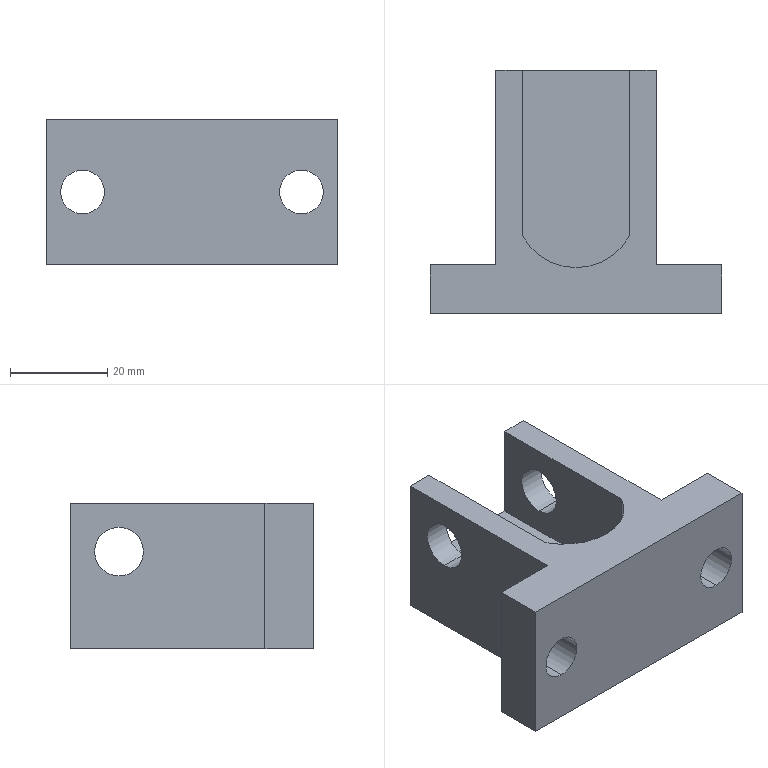Part | SolidWorks | features HoleWzd 3, ICE 3, Extrusion 1 | 1 solid | 22 faces | box 60 x 50 x 30 mm | volume 38448 mm3 | plane 13 | cylinder 9 | commonest cylinder face diameters 9 x4 10 x4 25 x1
STEP:
#1=CARTESIAN_POINT('',(13.5,40.,25.));
#2=VERTEX_POINT('',#1);
#3=CARTESIAN_POINT('',(13.5,40.,15.));
#4=VERTEX_POINT('',#3);
#5=CARTESIAN_POINT('',(13.5,40.,20.));
#6=DIRECTION('',(1.,0.,0.));
#7=DIRECTION('',(0.,1.,0.));
#8=AXIS2_PLACEMENT_3D('',#5,#6,#7);
#9=CIRCLE('',#8,5.);
#10=EDGE_CURVE('',#2,#4,#9,.T.);
#11=ORIENTED_EDGE('',*,*,#10,.F.);
#12=CARTESIAN_POINT('',(19.,40.,25.));
#13=VERTEX_POINT('',#12);
#14=CARTESIAN_POINT('',(19.,40.,25.));
#15=DIRECTION('',(1.,0.,0.));
#16=VECTOR('',#15,1000.);
#17=LINE('',#14,#16);
#18=EDGE_CURVE('',#2,#13,#17,.T.);
#19=ORIENTED_EDGE('',*,*,#18,.T.);
#20=CARTESIAN_POINT('',(19.,40.,15.));
#21=VERTEX_POINT('',#20);
#22=CARTESIAN_POINT('',(19.,40.,20.));
#23=DIRECTION('',(1.,0.,0.));
#24=DIRECTION('',(0.,0.,-1.));
#25=AXIS2_PLACEMENT_3D('',#22,#23,#24);
#26=CIRCLE('',#25,5.);
#27=EDGE_CURVE('',#13,#21,#26,.T.);
#28=ORIENTED_EDGE('',*,*,#27,.T.);
#29=CARTESIAN_POINT('',(19.,40.,15.));
#30=DIRECTION('',(1.,0.,0.));
#31=VECTOR('',#30,1000.);
#32=LINE('',#29,#31);
#33=EDGE_CURVE('',#4,#21,#32,.T.);
#34=ORIENTED_EDGE('',*,*,#33,.F.);
#35=EDGE_LOOP('',(#11,#19,#28,#34));
#36=FACE_OUTER_BOUND('',#35,.T.);
#37=CARTESIAN_POINT('',(19.,40.,20.));
#38=DIRECTION('',(1.,0.,0.));
#39=DIRECTION('',(0.,0.,-1.));
#40=AXIS2_PLACEMENT_3D('',#37,#38,#39);
#41=CYLINDRICAL_SURFACE('',#40,5.);
#42=ADVANCED_FACE('',(#36),#41,.F.);
#43=CARTESIAN_POINT('',(46.5,40.,15.));
#44=VERTEX_POINT('',#43);
#45=CARTESIAN_POINT('',(46.5,40.,25.));
#46=VERTEX_POINT('',#45);
#47=CARTESIAN_POINT('',(46.5,40.,20.));
#48=DIRECTION('',(-1.,0.,0.));
#49=DIRECTION('',(0.,0.,1.));
#50=AXIS2_PLACEMENT_3D('',#47,#48,#49);
#51=CIRCLE('',#50,5.);
#52=EDGE_CURVE('',#44,#46,#51,.T.);
#53=ORIENTED_EDGE('',*,*,#52,.F.);
#54=CARTESIAN_POINT('',(41.,40.,15.));
#55=VERTEX_POINT('',#54);
#56=CARTESIAN_POINT('',(41.,40.,15.));
#57=DIRECTION('',(-1.,0.,0.));
#58=VECTOR('',#57,1000.);
#59=LINE('',#56,#58);
#60=EDGE_CURVE('',#44,#55,#59,.T.);
#61=ORIENTED_EDGE('',*,*,#60,.T.);
#62=CARTESIAN_POINT('',(41.,40.,25.));
#63=VERTEX_POINT('',#62);
#64=CARTESIAN_POINT('',(41.,40.,20.));
#65=DIRECTION('',(-1.,0.,0.));
#66=DIRECTION('',(0.,0.,1.));
#67=AXIS2_PLACEMENT_3D('',#64,#65,#66);
#68=CIRCLE('',#67,5.);
#69=EDGE_CURVE('',#55,#63,#68,.T.);
#70=ORIENTED_EDGE('',*,*,#69,.T.);
#71=CARTESIAN_POINT('',(41.,40.,25.));
#72=DIRECTION('',(-1.,0.,0.));
#73=VECTOR('',#72,1000.);
#74=LINE('',#71,#73);
#75=EDGE_CURVE('',#46,#63,#74,.T.);
#76=ORIENTED_EDGE('',*,*,#75,.F.);
#77=EDGE_LOOP('',(#53,#61,#70,#76));
#78=FACE_OUTER_BOUND('',#77,.T.);
#79=CARTESIAN_POINT('',(41.,40.,20.));
#80=DIRECTION('',(-1.,0.,0.));
#81=DIRECTION('',(0.,0.,1.));
#82=AXIS2_PLACEMENT_3D('',#79,#80,#81);
#83=CYLINDRICAL_SURFACE('',#82,5.);
#84=ADVANCED_FACE('',(#78),#83,.F.);
#85=CARTESIAN_POINT('',(7.5,10.,19.5));
#86=VERTEX_POINT('',#85);
#87=CARTESIAN_POINT('',(7.5,10.,10.5));
#88=VERTEX_POINT('',#87);
#89=CARTESIAN_POINT('',(7.5,10.,15.));
#90=DIRECTION('',(0.,-1.,0.));
#91=DIRECTION('',(0.,0.,-1.));
#92=AXIS2_PLACEMENT_3D('',#89,#90,#91);
#93=CIRCLE('',#92,4.5);
#94=EDGE_CURVE('',#86,#88,#93,.T.);
#95=ORIENTED_EDGE('',*,*,#94,.F.);
#96=CARTESIAN_POINT('',(7.5,0.,19.5));
#97=VERTEX_POINT('',#96);
#98=CARTESIAN_POINT('',(7.5,0.,19.5));
#99=DIRECTION('',(0.,-1.,0.));
#100=VECTOR('',#99,1000.);
#101=LINE('',#98,#100);
#102=EDGE_CURVE('',#86,#97,#101,.T.);
#103=ORIENTED_EDGE('',*,*,#102,.T.);
#104=CARTESIAN_POINT('',(7.5,0.,10.5));
#105=VERTEX_POINT('',#104);
#106=CARTESIAN_POINT('',(7.5,0.,15.));
#107=DIRECTION('',(0.,-1.,0.));
#108=DIRECTION('',(0.,0.,-1.));
#109=AXIS2_PLACEMENT_3D('',#106,#107,#108);
#110=CIRCLE('',#109,4.5);
#111=EDGE_CURVE('',#97,#105,#110,.T.);
#112=ORIENTED_EDGE('',*,*,#111,.T.);
#113=CARTESIAN_POINT('',(7.5,0.,10.5));
#114=DIRECTION('',(0.,-1.,0.));
#115=VECTOR('',#114,1000.);
#116=LINE('',#113,#115);
#117=EDGE_CURVE('',#88,#105,#116,.T.);
#118=ORIENTED_EDGE('',*,*,#117,.F.);
#119=EDGE_LOOP('',(#95,#103,#112,#118));
#120=FACE_OUTER_BOUND('',#119,.T.);
#121=CARTESIAN_POINT('',(7.5,0.,15.));
#122=DIRECTION('',(0.,-1.,0.));
#123=DIRECTION('',(0.,0.,-1.));
#124=AXIS2_PLACEMENT_3D('',#121,#122,#123);
#125=CYLINDRICAL_SURFACE('',#124,4.5);
#126=ADVANCED_FACE('',(#120),#125,.F.);
#127=CARTESIAN_POINT('',(52.5,10.,19.5));
#128=VERTEX_POINT('',#127);
#129=CARTESIAN_POINT('',(52.5,10.,10.5));
#130=VERTEX_POINT('',#129);
#131=CARTESIAN_POINT('',(52.5,10.,15.));
#132=DIRECTION('',(0.,-1.,0.));
#133=DIRECTION('',(0.,0.,-1.));
#134=AXIS2_PLACEMENT_3D('',#131,#132,#133);
#135=CIRCLE('',#134,4.5);
#136=EDGE_CURVE('',#128,#130,#135,.T.);
#137=ORIENTED_EDGE('',*,*,#136,.F.);
#138=CARTESIAN_POINT('',(52.5,0.,19.5));
#139=VERTEX_POINT('',#138);
#140=CARTESIAN_POINT('',(52.5,0.,19.5));
#141=DIRECTION('',(0.,-1.,0.));
#142=VECTOR('',#141,1000.);
#143=LINE('',#140,#142);
#144=EDGE_CURVE('',#128,#139,#143,.T.);
#145=ORIENTED_EDGE('',*,*,#144,.T.);
#146=CARTESIAN_POINT('',(52.5,0.,10.5));
#147=VERTEX_POINT('',#146);
#148=CARTESIAN_POINT('',(52.5,0.,15.));
#149=DIRECTION('',(0.,-1.,0.));
#150=DIRECTION('',(0.,0.,-1.));
#151=AXIS2_PLACEMENT_3D('',#148,#149,#150);
#152=CIRCLE('',#151,4.5);
#153=EDGE_CURVE('',#139,#147,#152,.T.);
#154=ORIENTED_EDGE('',*,*,#153,.T.);
#155=CARTESIAN_POINT('',(52.5,0.,10.5));
#156=DIRECTION('',(0.,-1.,0.));
#157=VECTOR('',#156,1000.);
#158=LINE('',#155,#157);
#159=EDGE_CURVE('',#130,#147,#158,.T.);
#160=ORIENTED_EDGE('',*,*,#159,.F.);
#161=EDGE_LOOP('',(#137,#145,#154,#160));
#162=FACE_OUTER_BOUND('',#161,.T.);
#163=CARTESIAN_POINT('',(52.5,0.,15.));
#164=DIRECTION('',(0.,-1.,0.));
#165=DIRECTION('',(0.,0.,-1.));
#166=AXIS2_PLACEMENT_3D('',#163,#164,#165);
#167=CYLINDRICAL_SURFACE('',#166,4.5);
#168=ADVANCED_FACE('',(#162),#167,.F.);
#169=CARTESIAN_POINT('',(60.,10.,30.));
#170=VERTEX_POINT('',#169);
#171=CARTESIAN_POINT('',(60.,10.,0.));
#172=VERTEX_POINT('',#171);
#173=CARTESIAN_POINT('',(60.,10.,30.));
#174=DIRECTION('',(0.,0.,-1.));
#175=VECTOR('',#174,1000.);
#176=LINE('',#173,#175);
#177=EDGE_CURVE('',#170,#172,#176,.T.);
#178=ORIENTED_EDGE('',*,*,#177,.F.);
#179=CARTESIAN_POINT('',(60.,0.,30.));
#180=VERTEX_POINT('',#179);
#181=CARTESIAN_POINT('',(60.,0.,30.));
#182=DIRECTION('',(0.,1.,0.));
#183=VECTOR('',#182,1000.);
#184=LINE('',#181,#183);
#185=EDGE_CURVE('',#180,#170,#184,.T.);
#186=ORIENTED_EDGE('',*,*,#185,.F.);
#187=CARTESIAN_POINT('',(60.,0.,0.));
#188=VERTEX_POINT('',#187);
#189=CARTESIAN_POINT('',(60.,0.,0.));
#190=DIRECTION('',(0.,0.,1.));
#191=VECTOR('',#190,1000.);
#192=LINE('',#189,#191);
#193=EDGE_CURVE('',#188,#180,#192,.T.);
#194=ORIENTED_EDGE('',*,*,#193,.F.);
#195=CARTESIAN_POINT('',(60.,0.,0.));
#196=DIRECTION('',(0.,1.,0.));
#197=VECTOR('',#196,1000.);
#198=LINE('',#195,#197);
#199=EDGE_CURVE('',#188,#172,#198,.T.);
#200=ORIENTED_EDGE('',*,*,#199,.T.);
#201=EDGE_LOOP('',(#178,#186,#194,#200));
#202=FACE_OUTER_BOUND('',#201,.T.);
#203=CARTESIAN_POINT('',(60.,0.,0.));
#204=DIRECTION('',(1.,0.,0.));
#205=DIRECTION('',(0.,0.,-1.));
#206=AXIS2_PLACEMENT_3D('',#203,#204,#205);
#207=PLANE('',#206);
#208=ADVANCED_FACE('',(#202),#207,.T.);
#209=CARTESIAN_POINT('',(7.5,0.,15.));
#210=DIRECTION('',(0.,-1.,0.));
#211=DIRECTION('',(0.,0.,-1.));
#212=AXIS2_PLACEMENT_3D('',#209,#210,#211);
#213=CIRCLE('',#212,4.5);
#214=EDGE_CURVE('',#105,#97,#213,.T.);
#215=ORIENTED_EDGE('',*,*,#214,.F.);
#216=ORIENTED_EDGE('',*,*,#111,.F.);
#217=EDGE_LOOP('',(#215,#216));
#218=FACE_BOUND('',#217,.T.);
#219=CARTESIAN_POINT('',(52.5,0.,15.));
#220=DIRECTION('',(0.,-1.,0.));
#221=DIRECTION('',(0.,0.,-1.));
#222=AXIS2_PLACEMENT_3D('',#219,#220,#221);
#223=CIRCLE('',#222,4.5);
#224=EDGE_CURVE('',#147,#139,#223,.T.);
#225=ORIENTED_EDGE('',*,*,#224,.F.);
#226=ORIENTED_EDGE('',*,*,#153,.F.);
#227=EDGE_LOOP('',(#225,#226));
#228=FACE_BOUND('',#227,.T.);
#229=CARTESIAN_POINT('',(0.,0.,30.));
#230=VERTEX_POINT('',#229);
#231=CARTESIAN_POINT('',(0.,0.,30.));
#232=DIRECTION('',(1.,0.,0.));
#233=VECTOR('',#232,1000.);
#234=LINE('',#231,#233);
#235=EDGE_CURVE('',#230,#180,#234,.T.);
#236=ORIENTED_EDGE('',*,*,#235,.F.);
#237=CARTESIAN_POINT('',(0.,0.,0.));
#238=VERTEX_POINT('',#237);
#239=CARTESIAN_POINT('',(0.,0.,0.));
#240=DIRECTION('',(0.,0.,1.));
#241=VECTOR('',#240,1000.);
#242=LINE('',#239,#241);
#243=EDGE_CURVE('',#238,#230,#242,.T.);
#244=ORIENTED_EDGE('',*,*,#243,.F.);
#245=CARTESIAN_POINT('',(0.,0.,0.));
#246=DIRECTION('',(1.,0.,0.));
#247=VECTOR('',#246,1000.);
#248=LINE('',#245,#247);
#249=EDGE_CURVE('',#238,#188,#248,.T.);
#250=ORIENTED_EDGE('',*,*,#249,.T.);
#251=ORIENTED_EDGE('',*,*,#193,.T.);
#252=EDGE_LOOP('',(#236,#244,#250,#251));
#253=FACE_OUTER_BOUND('',#252,.T.);
#254=CARTESIAN_POINT('',(0.,0.,0.));
#255=DIRECTION('',(0.,-1.,0.));
#256=DIRECTION('',(0.,0.,-1.));
#257=AXIS2_PLACEMENT_3D('',#254,#255,#256);
#258=PLANE('',#257);
#259=ADVANCED_FACE('',(#218,#228,#253),#258,.T.);
#260=CARTESIAN_POINT('',(0.,10.,30.));
#261=VERTEX_POINT('',#260);
#262=CARTESIAN_POINT('',(0.,10.,0.));
#263=VERTEX_POINT('',#262);
#264=CARTESIAN_POINT('',(0.,10.,30.));
#265=DIRECTION('',(0.,0.,-1.));
#266=VECTOR('',#265,1000.);
#267=LINE('',#264,#266);
#268=EDGE_CURVE('',#261,#263,#267,.T.);
#269=ORIENTED_EDGE('',*,*,#268,.T.);
#270=CARTESIAN_POINT('',(0.,50.,0.));
#271=DIRECTION('',(0.,-1.,0.));
#272=VECTOR('',#271,1000.);
#273=LINE('',#270,#272);
#274=EDGE_CURVE('',#263,#238,#273,.T.);
#275=ORIENTED_EDGE('',*,*,#274,.T.);
#276=ORIENTED_EDGE('',*,*,#243,.T.);
#277=CARTESIAN_POINT('',(0.,50.,30.));
#278=DIRECTION('',(0.,-1.,0.));
#279=VECTOR('',#278,1000.);
#280=LINE('',#277,#279);
#281=EDGE_CURVE('',#261,#230,#280,.T.);
#282=ORIENTED_EDGE('',*,*,#281,.F.);
#283=EDGE_LOOP('',(#269,#275,#276,#282));
#284=FACE_OUTER_BOUND('',#283,.T.);
#285=CARTESIAN_POINT('',(0.,50.,0.));
#286=DIRECTION('',(-1.,0.,0.));
#287=DIRECTION('',(0.,0.,1.));
#288=AXIS2_PLACEMENT_3D('',#285,#286,#287);
#289=PLANE('',#288);
#290=ADVANCED_FACE('',(#284),#289,.T.);
#291=CARTESIAN_POINT('',(41.,50.,10.));
#292=VERTEX_POINT('',#291);
#293=CARTESIAN_POINT('',(41.,50.,30.));
#294=VERTEX_POINT('',#293);
#295=CARTESIAN_POINT('',(41.,50.,10.));
#296=DIRECTION('',(0.,0.,1.));
#297=VECTOR('',#296,1000.);
#298=LINE('',#295,#297);
#299=EDGE_CURVE('',#292,#294,#298,.T.);
#300=ORIENTED_EDGE('',*,*,#299,.T.);
#301=CARTESIAN_POINT('',(46.5,50.,30.));
#302=VERTEX_POINT('',#301);
#303=CARTESIAN_POINT('',(60.,50.,30.));
#304=DIRECTION('',(-1.,0.,0.));
#305=VECTOR('',#304,1000.);
#306=LINE('',#303,#305);
#307=EDGE_CURVE('',#302,#294,#306,.T.);
#308=ORIENTED_EDGE('',*,*,#307,.F.);
#309=CARTESIAN_POINT('',(46.5,50.,0.));
#310=VERTEX_POINT('',#309);
#311=CARTESIAN_POINT('',(46.5,50.,30.));
#312=DIRECTION('',(0.,0.,-1.));
#313=VECTOR('',#312,1000.);
#314=LINE('',#311,#313);
#315=EDGE_CURVE('',#302,#310,#314,.T.);
#316=ORIENTED_EDGE('',*,*,#315,.T.);
#317=CARTESIAN_POINT('',(13.5,50.,0.));
#318=VERTEX_POINT('',#317);
#319=CARTESIAN_POINT('',(60.,50.,0.));
#320=DIRECTION('',(-1.,0.,0.));
#321=VECTOR('',#320,1000.);
#322=LINE('',#319,#321);
#323=EDGE_CURVE('',#310,#318,#322,.T.);
#324=ORIENTED_EDGE('',*,*,#323,.T.);
#325=CARTESIAN_POINT('',(13.5,50.,30.));
#326=VERTEX_POINT('',#325);
#327=CARTESIAN_POINT('',(13.5,50.,30.));
#328=DIRECTION('',(0.,0.,-1.));
#329=VECTOR('',#328,1000.);
#330=LINE('',#327,#329);
#331=EDGE_CURVE('',#326,#318,#330,.T.);
#332=ORIENTED_EDGE('',*,*,#331,.F.);
#333=CARTESIAN_POINT('',(19.,50.,30.));
#334=VERTEX_POINT('',#333);
#335=CARTESIAN_POINT('',(60.,50.,30.));
#336=DIRECTION('',(-1.,0.,0.));
#337=VECTOR('',#336,1000.);
#338=LINE('',#335,#337);
#339=EDGE_CURVE('',#334,#326,#338,.T.);
#340=ORIENTED_EDGE('',*,*,#339,.F.);
#341=CARTESIAN_POINT('',(19.,50.,10.));
#342=VERTEX_POINT('',#341);
#343=CARTESIAN_POINT('',(19.,50.,10.));
#344=DIRECTION('',(0.,0.,1.));
#345=VECTOR('',#344,1000.);
#346=LINE('',#343,#345);
#347=EDGE_CURVE('',#342,#334,#346,.T.);
#348=ORIENTED_EDGE('',*,*,#347,.F.);
#349=CARTESIAN_POINT('',(41.,50.,10.));
#350=DIRECTION('',(-1.,0.,0.));
#351=VECTOR('',#350,1000.);
#352=LINE('',#349,#351);
#353=EDGE_CURVE('',#292,#342,#352,.T.);
#354=ORIENTED_EDGE('',*,*,#353,.F.);
#355=EDGE_LOOP('',(#300,#308,#316,#324,#332,#340,#348,#354));
#356=FACE_OUTER_BOUND('',#355,.T.);
#357=CARTESIAN_POINT('',(60.,50.,0.));
#358=DIRECTION('',(0.,1.,0.));
#359=DIRECTION('',(0.,0.,1.));
#360=AXIS2_PLACEMENT_3D('',#357,#358,#359);
#361=PLANE('',#360);
#362=ADVANCED_FACE('',(#356),#361,.T.);
#363=ORIENTED_EDGE('',*,*,#274,.F.);
#364=CARTESIAN_POINT('',(13.5,10.,0.));
#365=VERTEX_POINT('',#364);
#366=CARTESIAN_POINT('',(13.5,10.,0.));
#367=DIRECTION('',(-1.,0.,0.));
#368=VECTOR('',#367,1000.);
#369=LINE('',#366,#368);
#370=EDGE_CURVE('',#365,#263,#369,.T.);
#371=ORIENTED_EDGE('',*,*,#370,.F.);
#372=CARTESIAN_POINT('',(13.5,50.,0.));
#373=DIRECTION('',(0.,-1.,0.));
#374=VECTOR('',#373,1000.);
#375=LINE('',#372,#374);
#376=EDGE_CURVE('',#318,#365,#375,.T.);
#377=ORIENTED_EDGE('',*,*,#376,.F.);
#378=ORIENTED_EDGE('',*,*,#323,.F.);
#379=CARTESIAN_POINT('',(46.5,10.,0.));
#380=VERTEX_POINT('',#379);
#381=CARTESIAN_POINT('',(46.5,10.,0.));
#382=DIRECTION('',(0.,1.,0.));
#383=VECTOR('',#382,1000.);
#384=LINE('',#381,#383);
#385=EDGE_CURVE('',#380,#310,#384,.T.);
#386=ORIENTED_EDGE('',*,*,#385,.F.);
#387=CARTESIAN_POINT('',(60.,10.,0.));
#388=DIRECTION('',(-1.,0.,0.));
#389=VECTOR('',#388,1000.);
#390=LINE('',#387,#389);
#391=EDGE_CURVE('',#172,#380,#390,.T.);
#392=ORIENTED_EDGE('',*,*,#391,.F.);
#393=ORIENTED_EDGE('',*,*,#199,.F.);
#394=ORIENTED_EDGE('',*,*,#249,.F.);
#395=EDGE_LOOP('',(#363,#371,#377,#378,#386,#392,#393,#394));
#396=FACE_OUTER_BOUND('',#395,.T.);
#397=CARTESIAN_POINT('',(0.,0.,0.));
#398=DIRECTION('',(0.,0.,1.));
#399=DIRECTION('',(1.,0.,0.));
#400=AXIS2_PLACEMENT_3D('',#397,#398,#399);
#401=PLANE('',#400);
#402=ADVANCED_FACE('',(#396),#401,.F.);
#403=CARTESIAN_POINT('',(41.,16.,30.));
#404=VERTEX_POINT('',#403);
#405=CARTESIAN_POINT('',(41.,16.,30.));
#406=DIRECTION('',(0.,1.,0.));
#407=VECTOR('',#406,1000.);
#408=LINE('',#405,#407);
#409=EDGE_CURVE('',#404,#294,#408,.T.);
#410=ORIENTED_EDGE('',*,*,#409,.F.);
#411=CARTESIAN_POINT('',(19.,16.,30.));
#412=VERTEX_POINT('',#411);
#413=CARTESIAN_POINT('',(30.,21.937,30.));
#414=DIRECTION('',(0.,0.,1.));
#415=DIRECTION('',(1.,0.,0.));
#416=AXIS2_PLACEMENT_3D('',#413,#414,#415);
#417=CIRCLE('',#416,12.5);
#418=EDGE_CURVE('',#412,#404,#417,.T.);
#419=ORIENTED_EDGE('',*,*,#418,.F.);
#420=CARTESIAN_POINT('',(19.,50.,30.));
#421=DIRECTION('',(0.,-1.,0.));
#422=VECTOR('',#421,1000.);
#423=LINE('',#420,#422);
#424=EDGE_CURVE('',#334,#412,#423,.T.);
#425=ORIENTED_EDGE('',*,*,#424,.F.);
#426=ORIENTED_EDGE('',*,*,#339,.T.);
#427=CARTESIAN_POINT('',(13.5,10.,30.));
#428=VERTEX_POINT('',#427);
#429=CARTESIAN_POINT('',(13.5,50.,30.));
#430=DIRECTION('',(0.,-1.,0.));
#431=VECTOR('',#430,1000.);
#432=LINE('',#429,#431);
#433=EDGE_CURVE('',#326,#428,#432,.T.);
#434=ORIENTED_EDGE('',*,*,#433,.T.);
#435=CARTESIAN_POINT('',(13.5,10.,30.));
#436=DIRECTION('',(-1.,0.,0.));
#437=VECTOR('',#436,1000.);
#438=LINE('',#435,#437);
#439=EDGE_CURVE('',#428,#261,#438,.T.);
#440=ORIENTED_EDGE('',*,*,#439,.T.);
#441=ORIENTED_EDGE('',*,*,#281,.T.);
#442=ORIENTED_EDGE('',*,*,#235,.T.);
#443=ORIENTED_EDGE('',*,*,#185,.T.);
#444=CARTESIAN_POINT('',(46.5,10.,30.));
#445=VERTEX_POINT('',#444);
#446=CARTESIAN_POINT('',(60.,10.,30.));
#447=DIRECTION('',(-1.,0.,0.));
#448=VECTOR('',#447,1000.);
#449=LINE('',#446,#448);
#450=EDGE_CURVE('',#170,#445,#449,.T.);
#451=ORIENTED_EDGE('',*,*,#450,.T.);
#452=CARTESIAN_POINT('',(46.5,10.,30.));
#453=DIRECTION('',(0.,1.,0.));
#454=VECTOR('',#453,1000.);
#455=LINE('',#452,#454);
#456=EDGE_CURVE('',#445,#302,#455,.T.);
#457=ORIENTED_EDGE('',*,*,#456,.T.);
#458=ORIENTED_EDGE('',*,*,#307,.T.);
#459=EDGE_LOOP('',(#410,#419,#425,#426,#434,#440,#441,#442,#443,#451,#457,#458));
#460=FACE_OUTER_BOUND('',#459,.T.);
#461=CARTESIAN_POINT('',(0.,0.,30.));
#462=DIRECTION('',(0.,0.,1.));
#463=DIRECTION('',(1.,0.,0.));
#464=AXIS2_PLACEMENT_3D('',#461,#462,#463);
#465=PLANE('',#464);
#466=ADVANCED_FACE('',(#460),#465,.T.);
#467=CARTESIAN_POINT('',(46.5,40.,20.));
#468=DIRECTION('',(-1.,0.,0.));
#469=DIRECTION('',(0.,0.,1.));
#470=AXIS2_PLACEMENT_3D('',#467,#468,#469);
#471=CIRCLE('',#470,5.);
#472=EDGE_CURVE('',#46,#44,#471,.T.);
#473=ORIENTED_EDGE('',*,*,#472,.T.);
#474=ORIENTED_EDGE('',*,*,#52,.T.);
#475=EDGE_LOOP('',(#473,#474));
#476=FACE_BOUND('',#475,.T.);
#477=ORIENTED_EDGE('',*,*,#385,.T.);
#478=ORIENTED_EDGE('',*,*,#315,.F.);
#479=ORIENTED_EDGE('',*,*,#456,.F.);
#480=CARTESIAN_POINT('',(46.5,10.,30.));
#481=DIRECTION('',(0.,0.,-1.));
#482=VECTOR('',#481,1000.);
#483=LINE('',#480,#482);
#484=EDGE_CURVE('',#445,#380,#483,.T.);
#485=ORIENTED_EDGE('',*,*,#484,.T.);
#486=EDGE_LOOP('',(#477,#478,#479,#485));
#487=FACE_OUTER_BOUND('',#486,.T.);
#488=CARTESIAN_POINT('',(46.5,10.,30.));
#489=DIRECTION('',(-1.,0.,0.));
#490=DIRECTION('',(0.,0.,1.));
#491=AXIS2_PLACEMENT_3D('',#488,#489,#490);
#492=PLANE('',#491);
#493=ADVANCED_FACE('',(#476,#487),#492,.F.);
#494=CARTESIAN_POINT('',(52.5,10.,15.));
#495=DIRECTION('',(0.,-1.,0.));
#496=DIRECTION('',(0.,0.,-1.));
#497=AXIS2_PLACEMENT_3D('',#494,#495,#496);
#498=CIRCLE('',#497,4.5);
#499=EDGE_CURVE('',#130,#128,#498,.T.);
#500=ORIENTED_EDGE('',*,*,#499,.T.);
#501=ORIENTED_EDGE('',*,*,#136,.T.);
#502=EDGE_LOOP('',(#500,#501));
#503=FACE_BOUND('',#502,.T.);
#504=ORIENTED_EDGE('',*,*,#391,.T.);
#505=ORIENTED_EDGE('',*,*,#484,.F.);
#506=ORIENTED_EDGE('',*,*,#450,.F.);
#507=ORIENTED_EDGE('',*,*,#177,.T.);
#508=EDGE_LOOP('',(#504,#505,#506,#507));
#509=FACE_OUTER_BOUND('',#508,.T.);
#510=CARTESIAN_POINT('',(60.,10.,30.));
#511=DIRECTION('',(0.,-1.,0.));
#512=DIRECTION('',(0.,0.,-1.));
#513=AXIS2_PLACEMENT_3D('',#510,#511,#512);
#514=PLANE('',#513);
#515=ADVANCED_FACE('',(#503,#509),#514,.F.);
#516=CARTESIAN_POINT('',(7.5,10.,15.));
#517=DIRECTION('',(0.,-1.,0.));
#518=DIRECTION('',(0.,0.,-1.));
#519=AXIS2_PLACEMENT_3D('',#516,#517,#518);
#520=CIRCLE('',#519,4.5);
#521=EDGE_CURVE('',#88,#86,#520,.T.);
#522=ORIENTED_EDGE('',*,*,#521,.T.);
#523=ORIENTED_EDGE('',*,*,#94,.T.);
#524=EDGE_LOOP('',(#522,#523));
#525=FACE_BOUND('',#524,.T.);
#526=ORIENTED_EDGE('',*,*,#370,.T.);
#527=ORIENTED_EDGE('',*,*,#268,.F.);
#528=ORIENTED_EDGE('',*,*,#439,.F.);
#529=CARTESIAN_POINT('',(13.5,10.,30.));
#530=DIRECTION('',(0.,0.,-1.));
#531=VECTOR('',#530,1000.);
#532=LINE('',#529,#531);
#533=EDGE_CURVE('',#428,#365,#532,.T.);
#534=ORIENTED_EDGE('',*,*,#533,.T.);
#535=EDGE_LOOP('',(#526,#527,#528,#534));
#536=FACE_OUTER_BOUND('',#535,.T.);
#537=CARTESIAN_POINT('',(13.5,10.,30.));
#538=DIRECTION('',(0.,-1.,0.));
#539=DIRECTION('',(0.,0.,-1.));
#540=AXIS2_PLACEMENT_3D('',#537,#538,#539);
#541=PLANE('',#540);
#542=ADVANCED_FACE('',(#525,#536),#541,.F.);
#543=CARTESIAN_POINT('',(13.5,40.,20.));
#544=DIRECTION('',(1.,0.,0.));
#545=DIRECTION('',(0.,1.,0.));
#546=AXIS2_PLACEMENT_3D('',#543,#544,#545);
#547=CIRCLE('',#546,5.);
#548=EDGE_CURVE('',#4,#2,#547,.T.);
#549=ORIENTED_EDGE('',*,*,#548,.T.);
#550=ORIENTED_EDGE('',*,*,#10,.T.);
#551=EDGE_LOOP('',(#549,#550));
#552=FACE_BOUND('',#551,.T.);
#553=ORIENTED_EDGE('',*,*,#376,.T.);
#554=ORIENTED_EDGE('',*,*,#533,.F.);
#555=ORIENTED_EDGE('',*,*,#433,.F.);
#556=ORIENTED_EDGE('',*,*,#331,.T.);
#557=EDGE_LOOP('',(#553,#554,#555,#556));
#558=FACE_OUTER_BOUND('',#557,.T.);
#559=CARTESIAN_POINT('',(13.5,50.,30.));
#560=DIRECTION('',(1.,0.,0.));
#561=DIRECTION('',(0.,1.,0.));
#562=AXIS2_PLACEMENT_3D('',#559,#560,#561);
#563=PLANE('',#562);
#564=ADVANCED_FACE('',(#552,#558),#563,.F.);
#565=CARTESIAN_POINT('',(41.,40.,20.));
#566=DIRECTION('',(-1.,0.,0.));
#567=DIRECTION('',(0.,0.,1.));
#568=AXIS2_PLACEMENT_3D('',#565,#566,#567);
#569=CIRCLE('',#568,5.);
#570=EDGE_CURVE('',#63,#55,#569,.T.);
#571=ORIENTED_EDGE('',*,*,#570,.F.);
#572=ORIENTED_EDGE('',*,*,#69,.F.);
#573=EDGE_LOOP('',(#571,#572));
#574=FACE_BOUND('',#573,.T.);
#575=ORIENTED_EDGE('',*,*,#409,.T.);
#576=ORIENTED_EDGE('',*,*,#299,.F.);
#577=CARTESIAN_POINT('',(41.,16.,10.));
#578=VERTEX_POINT('',#577);
#579=CARTESIAN_POINT('',(41.,16.,10.));
#580=DIRECTION('',(0.,1.,0.));
#581=VECTOR('',#580,1000.);
#582=LINE('',#579,#581);
#583=EDGE_CURVE('',#578,#292,#582,.T.);
#584=ORIENTED_EDGE('',*,*,#583,.F.);
#585=CARTESIAN_POINT('',(41.,16.,10.));
#586=DIRECTION('',(0.,0.,1.));
#587=VECTOR('',#586,1000.);
#588=LINE('',#585,#587);
#589=EDGE_CURVE('',#578,#404,#588,.T.);
#590=ORIENTED_EDGE('',*,*,#589,.T.);
#591=EDGE_LOOP('',(#575,#576,#584,#590));
#592=FACE_OUTER_BOUND('',#591,.T.);
#593=CARTESIAN_POINT('',(41.,16.,10.));
#594=DIRECTION('',(1.,0.,0.));
#595=DIRECTION('',(0.,1.,0.));
#596=AXIS2_PLACEMENT_3D('',#593,#594,#595);
#597=PLANE('',#596);
#598=ADVANCED_FACE('',(#574,#592),#597,.F.);
#599=ORIENTED_EDGE('',*,*,#418,.T.);
#600=ORIENTED_EDGE('',*,*,#589,.F.);
#601=CARTESIAN_POINT('',(19.,16.,10.));
#602=VERTEX_POINT('',#601);
#603=CARTESIAN_POINT('',(30.,21.937,10.));
#604=DIRECTION('',(0.,0.,1.));
#605=DIRECTION('',(1.,0.,0.));
#606=AXIS2_PLACEMENT_3D('',#603,#604,#605);
#607=CIRCLE('',#606,12.5);
#608=EDGE_CURVE('',#602,#578,#607,.T.);
#609=ORIENTED_EDGE('',*,*,#608,.F.);
#610=CARTESIAN_POINT('',(19.,16.,10.));
#611=DIRECTION('',(0.,0.,1.));
#612=VECTOR('',#611,1000.);
#613=LINE('',#610,#612);
#614=EDGE_CURVE('',#602,#412,#613,.T.);
#615=ORIENTED_EDGE('',*,*,#614,.T.);
#616=EDGE_LOOP('',(#599,#600,#609,#615));
#617=FACE_OUTER_BOUND('',#616,.T.);
#618=CARTESIAN_POINT('',(30.,21.937,10.));
#619=DIRECTION('',(0.,0.,1.));
#620=DIRECTION('',(1.,0.,0.));
#621=AXIS2_PLACEMENT_3D('',#618,#619,#620);
#622=CYLINDRICAL_SURFACE('',#621,12.5);
#623=ADVANCED_FACE('',(#617),#622,.F.);
#624=CARTESIAN_POINT('',(19.,40.,20.));
#625=DIRECTION('',(1.,0.,0.));
#626=DIRECTION('',(0.,0.,-1.));
#627=AXIS2_PLACEMENT_3D('',#624,#625,#626);
#628=CIRCLE('',#627,5.);
#629=EDGE_CURVE('',#21,#13,#628,.T.);
#630=ORIENTED_EDGE('',*,*,#629,.F.);
#631=ORIENTED_EDGE('',*,*,#27,.F.);
#632=EDGE_LOOP('',(#630,#631));
#633=FACE_BOUND('',#632,.T.);
#634=ORIENTED_EDGE('',*,*,#424,.T.);
#635=ORIENTED_EDGE('',*,*,#614,.F.);
#636=CARTESIAN_POINT('',(19.,50.,10.));
#637=DIRECTION('',(0.,-1.,0.));
#638=VECTOR('',#637,1000.);
#639=LINE('',#636,#638);
#640=EDGE_CURVE('',#342,#602,#639,.T.);
#641=ORIENTED_EDGE('',*,*,#640,.F.);
#642=ORIENTED_EDGE('',*,*,#347,.T.);
#643=EDGE_LOOP('',(#634,#635,#641,#642));
#644=FACE_OUTER_BOUND('',#643,.T.);
#645=CARTESIAN_POINT('',(19.,50.,10.));
#646=DIRECTION('',(-1.,0.,0.));
#647=DIRECTION('',(0.,-1.,0.));
#648=AXIS2_PLACEMENT_3D('',#645,#646,#647);
#649=PLANE('',#648);
#650=ADVANCED_FACE('',(#633,#644),#649,.F.);
#651=ORIENTED_EDGE('',*,*,#353,.T.);
#652=ORIENTED_EDGE('',*,*,#640,.T.);
#653=ORIENTED_EDGE('',*,*,#608,.T.);
#654=ORIENTED_EDGE('',*,*,#583,.T.);
#655=EDGE_LOOP('',(#651,#652,#653,#654));
#656=FACE_OUTER_BOUND('',#655,.T.);
#657=CARTESIAN_POINT('',(30.,21.937,10.));
#658=DIRECTION('',(0.,0.,1.));
#659=DIRECTION('',(1.,0.,0.));
#660=AXIS2_PLACEMENT_3D('',#657,#658,#659);
#661=PLANE('',#660);
#662=ADVANCED_FACE('',(#656),#661,.T.);
#663=ORIENTED_EDGE('',*,*,#144,.F.);
#664=ORIENTED_EDGE('',*,*,#499,.F.);
#665=ORIENTED_EDGE('',*,*,#159,.T.);
#666=ORIENTED_EDGE('',*,*,#224,.T.);
#667=EDGE_LOOP('',(#663,#664,#665,#666));
#668=FACE_OUTER_BOUND('',#667,.T.);
#669=CARTESIAN_POINT('',(52.5,0.,15.));
#670=DIRECTION('',(0.,-1.,0.));
#671=DIRECTION('',(0.,0.,-1.));
#672=AXIS2_PLACEMENT_3D('',#669,#670,#671);
#673=CYLINDRICAL_SURFACE('',#672,4.5);
#674=ADVANCED_FACE('',(#668),#673,.F.);
#675=ORIENTED_EDGE('',*,*,#102,.F.);
#676=ORIENTED_EDGE('',*,*,#521,.F.);
#677=ORIENTED_EDGE('',*,*,#117,.T.);
#678=ORIENTED_EDGE('',*,*,#214,.T.);
#679=EDGE_LOOP('',(#675,#676,#677,#678));
#680=FACE_OUTER_BOUND('',#679,.T.);
#681=CARTESIAN_POINT('',(7.5,0.,15.));
#682=DIRECTION('',(0.,-1.,0.));
#683=DIRECTION('',(0.,0.,-1.));
#684=AXIS2_PLACEMENT_3D('',#681,#682,#683);
#685=CYLINDRICAL_SURFACE('',#684,4.5);
#686=ADVANCED_FACE('',(#680),#685,.F.);
#687=ORIENTED_EDGE('',*,*,#60,.F.);
#688=ORIENTED_EDGE('',*,*,#472,.F.);
#689=ORIENTED_EDGE('',*,*,#75,.T.);
#690=ORIENTED_EDGE('',*,*,#570,.T.);
#691=EDGE_LOOP('',(#687,#688,#689,#690));
#692=FACE_OUTER_BOUND('',#691,.T.);
#693=CARTESIAN_POINT('',(41.,40.,20.));
#694=DIRECTION('',(-1.,0.,0.));
#695=DIRECTION('',(0.,0.,1.));
#696=AXIS2_PLACEMENT_3D('',#693,#694,#695);
#697=CYLINDRICAL_SURFACE('',#696,5.);
#698=ADVANCED_FACE('',(#692),#697,.F.);
#699=ORIENTED_EDGE('',*,*,#18,.F.);
#700=ORIENTED_EDGE('',*,*,#548,.F.);
#701=ORIENTED_EDGE('',*,*,#33,.T.);
#702=ORIENTED_EDGE('',*,*,#629,.T.);
#703=EDGE_LOOP('',(#699,#700,#701,#702));
#704=FACE_OUTER_BOUND('',#703,.T.);
#705=CARTESIAN_POINT('',(19.,40.,20.));
#706=DIRECTION('',(1.,0.,0.));
#707=DIRECTION('',(0.,0.,-1.));
#708=AXIS2_PLACEMENT_3D('',#705,#706,#707);
#709=CYLINDRICAL_SURFACE('',#708,5.);
#710=ADVANCED_FACE('',(#704),#709,.F.);
#711=CLOSED_SHELL('',(#42,#84,#126,#168,#208,#259,#290,#362,#402,#466,#493,#515,#542,#564,#598,#623,#650,#662,#674,#686,#698,#710));
#712=MANIFOLD_SOLID_BREP('',#711);
#713=CARTESIAN_POINT('',(0.,0.,0.));
#714=DIRECTION('',(0.,0.,1.));
#715=DIRECTION('',(1.,0.,0.));
#716=AXIS2_PLACEMENT_3D('',#713,#714,#715);
#717=(LENGTH_UNIT()NAMED_UNIT(*)SI_UNIT(.MILLI.,.METRE.));
#718=UNCERTAINTY_MEASURE_WITH_UNIT(LENGTH_MEASURE(0.00001),#717,'','');
#719=(NAMED_UNIT(*)PLANE_ANGLE_UNIT()SI_UNIT($,.RADIAN.));
#720=(NAMED_UNIT(*)SI_UNIT($,.STERADIAN.)SOLID_ANGLE_UNIT());
#721=(GEOMETRIC_REPRESENTATION_CONTEXT(3)GLOBAL_UNCERTAINTY_ASSIGNED_CONTEXT((#718))GLOBAL_UNIT_ASSIGNED_CONTEXT((#717,#719,#720))REPRESENTATION_CONTEXT('',''));
#722=ADVANCED_BREP_SHAPE_REPRESENTATION('',(#712,#716),#721);